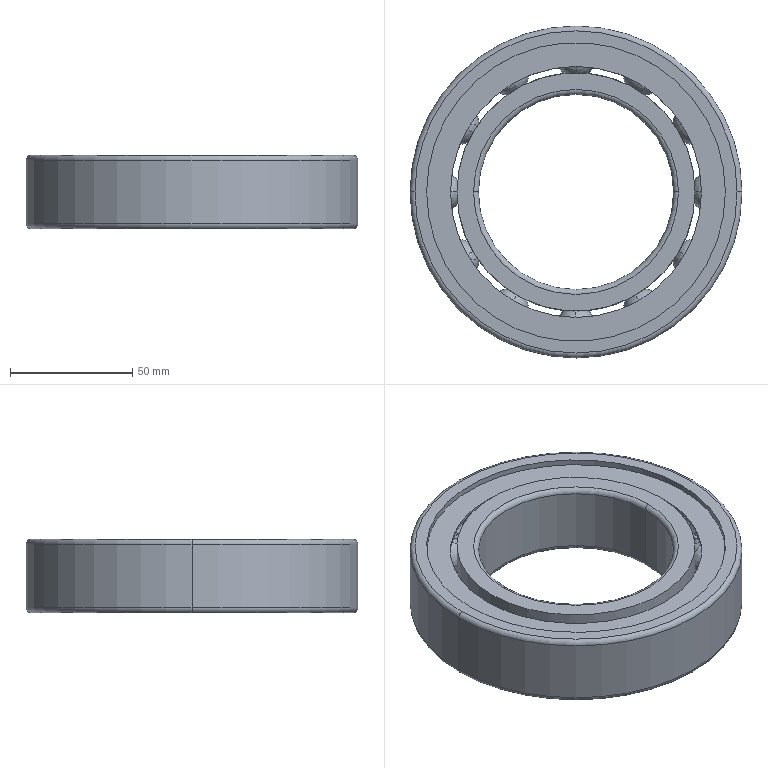Part | SolidWorks | features BaseBody 1 | 1 solid | 296 faces | box 136 x 136 x 30 mm | volume 181462 mm3 | sphere 196 | torus 44 | plane 32 | cylinder 24 | commonest cylinder face diameters 122.4 x8 97.6 x4 102.88 x4 80 x2 108.69 x2 111.31 x2